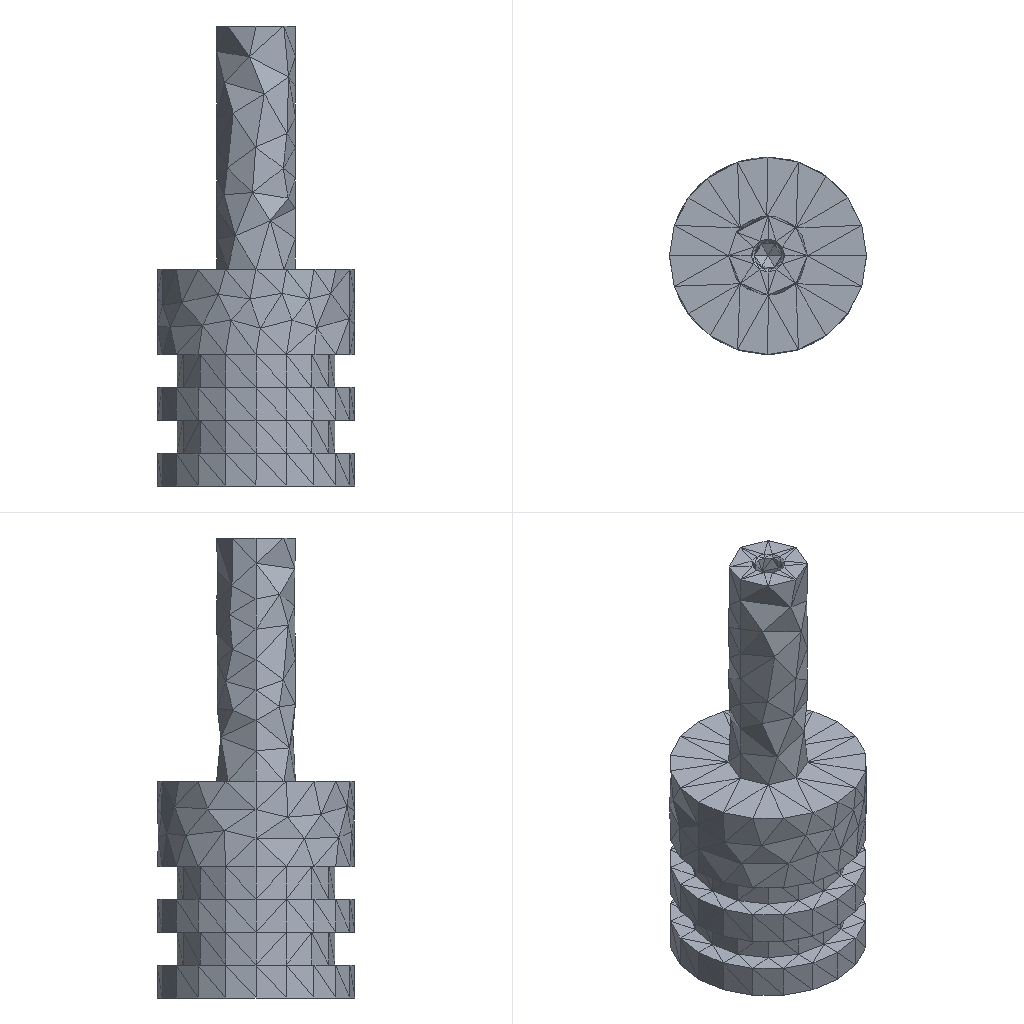Simulation study | ansys workbench
Ansys APDL input file, long lists of numbers shortened:
/batch
/config,noeldb,1     ! force off writing results to database
*get,_wallstrt,active,,time,wall
! ANSYS input file written by Workbench version 2022 R1
! File used for geometry attach: F:\ansys（分析文件汇总)\ansys刀片有限元分析\装配体\轴.STEP
/title,2222--____ (F5)
! ****** Begin Custom Load Command Snippet ******
/COM, ACT Extensions:
/COM,     LSDYNA, 2021.1
/COM,
! ****** End   Custom Load Command Snippet ******
*DIM,_wb_ProjectScratch_dir,string,248
_wb_ProjectScratch_dir(1) = 'F:\ansys（分析文件汇总)\ansys刀片有限元分析\_ProjectScratch\ScrD8CE\'
*DIM,_wb_SolverFiles_dir,string,248
_wb_SolverFiles_dir(1) = 'F:\ansys（分析文件汇总)\ansys刀片有限元分析\2222_files\dp0\SYS-3\MECH\'
*DIM,_wb_userfiles_dir,string,248
_wb_userfiles_dir(1) = 'F:\ansys（分析文件汇总)\ansys刀片有限元分析\2222_files\user_files\'
/com,--- Data in consistent NMM units. See Solving Units in the help system for more information.
/units,MPA
/nopr
/wb,file,start              !  signify a WB generated input file
/prep7
! Turn off shape checking because checks already performed inside WB mesher.
! See help system for more information.
SHPP,OFF,,NOWARN
/nolist
etcon,set             ! allow ANSYS to choose best KEYOP's for 180x elements, resets any applicable keyopt to MAPDL defaults
/com,*********** Nodes for the whole assembly ***********
nblock,3,,2839
(1i9,3e20.9e3)
        1     1.500000000E+01     1.836970199E-15     3.300000000E+01
! (2580 more lines like these left out)
-1
/com,*********** Nodes for all Remote Points ***********
nblock,3
(1i9,3e20.9e3)
     2582     1.856511411E-16     0.000000000E+00     3.780905181E+01
-1
/wb,elem,start            !  set before creation of elements
/com,*********** Elements for Body 1 "_-FreeParts|____(____)1" ***********
et,1,187
eblock,19,solid,,1357
(19i9)
        1        1        1        1        0        0        0        0       10        0        1       27      273       56      429      579      798      577      583
! (2713 more lines like these left out)
-1
/wb,elem,end               !  done creating elements
/com,*********** Send User Defined Coordinate System(s) ***********
csys,0
toffst,273.15,  ! Temperature offset from absolute zero
/com,*********** Set Reference Temperature ***********
tref,22.
/wb,mat,start              !  starting to send materials
/com,*********** Send Materials ***********
Temperature = 'TEMP' ! Temperature
MP,DENS,1,7.85e-09,	! tonne mm^-3
MP,ALPX,1,1.2e-05,	! C^-1
MP,C,1,434000000,	! mm^2 s^-2 C^-1
MP,KXX,1,60.5,	! tonne mm s^-3 C^-1
MP,RSVX,1,0.00017,	! ohm mm
MP,EX,1,200000,	! tonne s^-2 mm^-1
MP,NUXY,1,0.3,
MP,MURX,1,10000,
/wb,mat,end                !  done sending materials
!************************* Model Summary ********************
!_-FreeParts|____(____)1,	结构钢,	matid,	1
!************************* End Model Summary ********************
! get the diagonal of the bounding box. Needed later for other things
*get,_xmin,node,,mnloc,x
*get,_ymin,node,,mnloc,y
*get,_zmin,node,,mnloc,z
*get,_xmax,node,,mxloc,x
*get,_ymax,node,,mxloc,y
*get,_zmax,node,,mxloc,z
_ASMDIAG=(_xmax-_xmin)*(_xmax-_xmin)+(_ymax-_ymin)*(_ymax-_ymin)+(_zmax-_zmin)*(_zmax-_zmin)
_ASMDIAG=SQRT(_ASMDIAG)
/wb,contact,start          !  starting to send contact
/wb,contact,end            !  done creating contacts
/golist
/wb,load,start             !  starting to send loads
/com,*********** Fixed Supports ***********
CMBLOCK,_FIXEDSU,NODE,      274
(8i10)
        51        52        53        54        59        60        61        62
! (34 more lines like these left out)
cmsel,s,_FIXEDSU
d,all,all
nsel,all
/com,*********** Create Remote Point "内部远程点" ***********
! -------- Remote Point Used by "力矩" --------
*set,tid,3
*set,cid,2
et,cid,174
et,tid,170
keyo,tid,2,1               ! Don't fix the pilot node
keyo,tid,4,111111
keyo,cid,12,5              ! Bonded Contact
keyo,cid,4,1               ! Deformable RBE3 style load
keyo,cid,2,2               ! MPC style contact
eblock,10,,,170
(15i9)
     2089        2        2        2        0       29       27       33       33      575      576       33      593
! (169 more lines like these left out)
-1
*set,_npilot,2582
_npilot33=_npilot
type,tid
mat ,cid
real,cid
tshape,pilo
en,2259,_npilot
tshape
/com,*********** Construct Moment Using Remote Attachment ***********
/gst,on,on
fini
*get,_numnode,node,0,count
*get,_numelem,elem,0,count
*get, _MAXELEMNUM, elem, 0, NUM, MAX
*get, _MAXNODENUM, node, 0, NUM, MAX
*get, _MAXELEMTYPE, etyp, 0, NUM, MAX
*get, _MAXREALCONST, real, 0, NUM, MAX
/go
/wb,load,end               !  done creating loads
/com,--- Number of total nodes = %_numnode%
/com,--- Number of contact elements = 170
/com,--- Number of spring elements = 0
/com,--- Number of bearing elements = 0
/com,--- Number of solid elements = 1357
/com,--- Number of condensed parts = 0
/com,--- Number of total elements = %_numelem%
*get,_wallbsol,active,,time,wall
/com,****************************************************************************
/com,*************************    SOLUTION       ********************************
/com,****************************************************************************
/solu
antype,0                   ! static analysis
_thickRatio=  0     ! Ratio of thick parts in the model
eqsl,sparse,,,,,1
cntr,print,1               ! print out contact info and also make no initial contact an error
dmpoption,emat,no             ! Don't combine emat file for DANSYS
dmpoption,esav,no             ! Don't combine esav file for DANSYS
nldiag,cont,iter           ! print out contact info each equilibrium iteration
rescontrol,,none                 ! Do not keep any restart files
/com,****************************************************
/com,******************* SOLVE FOR LS 1 OF 1 ****************
nsel,s,node,,2582
f,all,mx,0.
f,all,my,0.
f,all,mz,52000.
nsel,all
/nopr
/gopr
nsub,1,1,1
time,1.
outres,erase
outres,all,none
outres,nsol,all,
outres,rsol,all
outres,eangl,all
outres,etmp,all
outres,veng,all
outres,strs,all,
outres,epel,all,
outres,eppl,all,
outres,cont,all,
! *********** WB SOLVE COMMAND ***********
! check interactive state
*get,ANSINTER_,active,,int
*if,ANSINTER_,ne,0,then
/eof
*endif
solve
/com *************** Write FE CONNECTORS *********
CEWRITE,file,ce,,INTE
/com,****************************************************
/com,*************** FINISHED SOLVE FOR LS 1 *************
*get,_wallasol,active,,time,wall
/nopr
*get,_numnode,node,0,count
*get,_numelem,elem,0,count
*get, _MAXELEMNUM, elem, 0, NUM, MAX
*get, _MAXNODENUM, node, 0, NUM, MAX,,,INTERNAL
*get, _MAXELEMTYPE, etyp, 0, NUM, MAX
*get, _MAXREALCONST, real, 0, NUM, MAX
/gopr
/post1
xmlo,ENCODING,ISO-8859-1
xmlo,parm
/xml,parm,xml
fini
/gopr
*get,_walldone,active,,time,wall
_preptime=(_wallbsol-_wallstrt)*3600
_solvtime=(_wallasol-_wallbsol)*3600
_posttime=(_walldone-_wallasol)*3600
_totaltim=(_walldone-_wallstrt)*3600
*get,_dlbratio,active,0,solu,dlbr
*get,_combtime,active,0,solu,comb
*get,_ssmode,active,0,solu,ssmm
*get,_ndofs,active,0,solu,ndof
*get,_sol_end_time,active,0,set,time
*if,_sol_end_time,eq,1.,then
/fclean				!clean distributed files
*endif
/com,--- Total number of nodes = %_numnode%
/com,--- Total number of elements = %_numelem%
/com,--- Element load balance ratio = %_dlbratio%
/com,--- Time to combine distributed files = %_combtime%
/com,--- Sparse memory mode = %_ssmode%
/com,--- Number of DOF = %_ndofs%
/wb,file,end               ! done with WB generated input